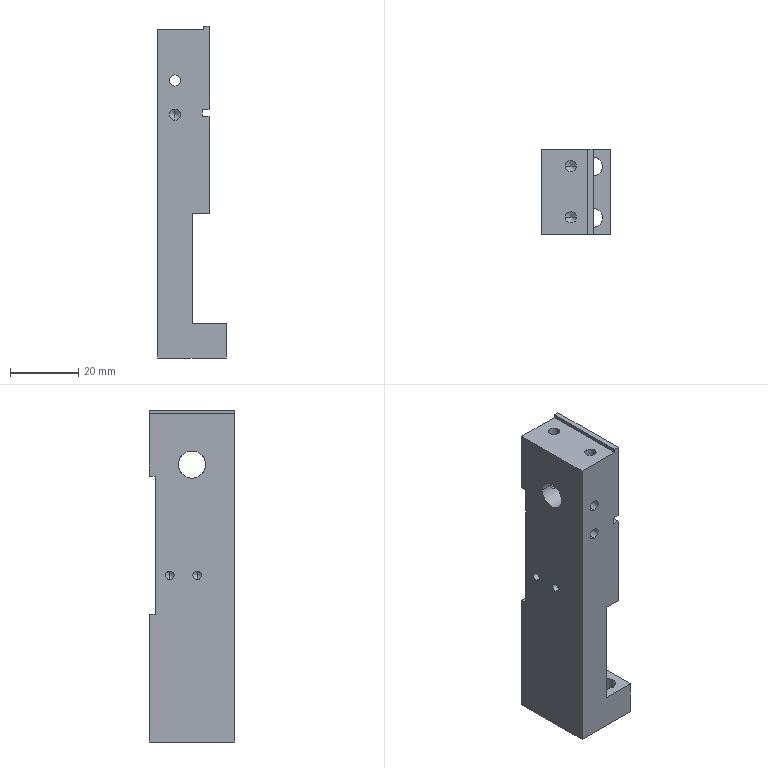Part | STEP file | 11-FG-B00111 | 1 solid | 66 faces | box 20 x 25 x 97.4 mm | volume 30314 mm3 | cylinder 28 | plane 20 | cone 18 | commonest cylinder face diameters 3.3 x14 2.5 x8 5.5 x4 8 x2